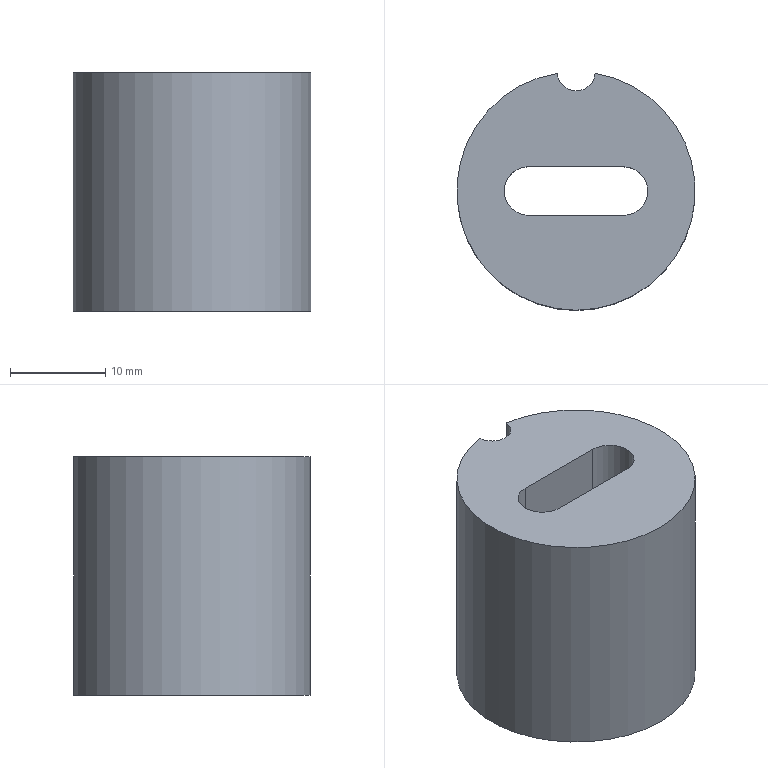Part | NX | features solid 2 | 1 solid | 10 faces | box 25 x 24.842 x 25 mm | volume 7869 mm3 | cylinder 5 | plane 5 | commonest cylinder face diameters 5.1 x2 4 x1 16.6 x1 25 x1
STEP:
#1=CARTESIAN_POINT('',(-200.99,448.658,32.));
#2=VERTEX_POINT('',#1);
#3=CARTESIAN_POINT('',(-200.99,448.658,57.));
#4=VERTEX_POINT('',#3);
#5=CARTESIAN_POINT('',(-200.99,448.658,44.5));
#6=DIRECTION('',(0.,0.,1.));
#7=VECTOR('',#6,1000.);
#8=LINE('',#5,#7);
#9=EDGE_CURVE('',#2,#4,#8,.T.);
#10=ORIENTED_EDGE('',*,*,#9,.T.);
#11=CARTESIAN_POINT('',(-204.978,448.663,57.));
#12=VERTEX_POINT('',#11);
#13=CARTESIAN_POINT('',(-202.998,436.321,57.));
#14=DIRECTION('',(0.,0.,-1.));
#15=DIRECTION('',(0.001167,1.,0.));
#16=AXIS2_PLACEMENT_3D('',#13,#14,#15);
#17=CIRCLE('',#16,12.5);
#18=EDGE_CURVE('',#4,#12,#17,.T.);
#19=ORIENTED_EDGE('',*,*,#18,.T.);
#20=CARTESIAN_POINT('',(-204.978,448.663,32.));
#21=VERTEX_POINT('',#20);
#22=CARTESIAN_POINT('',(-204.978,448.663,44.5));
#23=DIRECTION('',(0.,0.,1.));
#24=VECTOR('',#23,1000.);
#25=LINE('',#22,#24);
#26=EDGE_CURVE('',#12,#21,#25,.F.);
#27=ORIENTED_EDGE('',*,*,#26,.T.);
#28=CARTESIAN_POINT('',(-202.998,436.321,32.));
#29=DIRECTION('',(0.,0.,-1.));
#30=DIRECTION('',(0.001167,1.,0.));
#31=AXIS2_PLACEMENT_3D('',#28,#29,#30);
#32=CIRCLE('',#31,12.5);
#33=EDGE_CURVE('',#2,#21,#32,.T.);
#34=ORIENTED_EDGE('',*,*,#33,.F.);
#35=EDGE_LOOP('',(#10,#19,#27,#34));
#36=FACE_BOUND('',#35,.T.);
#37=CARTESIAN_POINT('',(-202.998,436.321,32.));
#38=DIRECTION('',(0.,0.,1.));
#39=DIRECTION('',(0.001167,1.,0.));
#40=AXIS2_PLACEMENT_3D('',#37,#38,#39);
#41=CYLINDRICAL_SURFACE('',#40,12.5);
#42=ADVANCED_FACE('',(#36),#41,.T.);
#43=CARTESIAN_POINT('',(-202.989,444.621,32.));
#44=VERTEX_POINT('',#43);
#45=CARTESIAN_POINT('',(-202.998,436.321,32.));
#46=DIRECTION('',(0.,0.,-1.));
#47=DIRECTION('',(0.001167,1.,0.));
#48=AXIS2_PLACEMENT_3D('',#45,#46,#47);
#49=CIRCLE('',#48,8.3);
#50=EDGE_CURVE('',#44,#44,#49,.T.);
#51=ORIENTED_EDGE('',*,*,#50,.F.);
#52=EDGE_LOOP('',(#51));
#53=FACE_BOUND('',#52,.T.);
#54=ORIENTED_EDGE('',*,*,#33,.T.);
#55=CARTESIAN_POINT('',(-202.984,448.821,32.));
#56=DIRECTION('',(0.,0.,-1.));
#57=DIRECTION('',(0.001167,1.,0.));
#58=AXIS2_PLACEMENT_3D('',#55,#56,#57);
#59=CIRCLE('',#58,2.);
#60=EDGE_CURVE('',#2,#21,#59,.T.);
#61=ORIENTED_EDGE('',*,*,#60,.F.);
#62=EDGE_LOOP('',(#54,#61));
#63=FACE_BOUND('',#62,.T.);
#64=CARTESIAN_POINT('',(-202.998,436.321,32.));
#65=DIRECTION('',(0.,0.,1.));
#66=DIRECTION('',(0.001167,1.,0.));
#67=AXIS2_PLACEMENT_3D('',#64,#65,#66);
#68=PLANE('',#67);
#69=ADVANCED_FACE('',(#53,#63),#68,.F.);
#70=CARTESIAN_POINT('',(-198.001,433.765,57.));
#71=VERTEX_POINT('',#70);
#72=CARTESIAN_POINT('',(-208.001,433.777,57.));
#73=VERTEX_POINT('',#72);
#74=CARTESIAN_POINT('',(-198.001,433.765,57.));
#75=DIRECTION('',(-1.,0.001167,0.));
#76=VECTOR('',#75,1000.);
#77=LINE('',#74,#76);
#78=EDGE_CURVE('',#71,#73,#77,.T.);
#79=ORIENTED_EDGE('',*,*,#78,.T.);
#80=CARTESIAN_POINT('',(-207.995,438.877,57.));
#81=VERTEX_POINT('',#80);
#82=CARTESIAN_POINT('',(-207.998,436.327,57.));
#83=DIRECTION('',(0.,0.,-1.));
#84=DIRECTION('',(0.001167,1.,0.));
#85=AXIS2_PLACEMENT_3D('',#82,#83,#84);
#86=CIRCLE('',#85,2.55);
#87=EDGE_CURVE('',#73,#81,#86,.T.);
#88=ORIENTED_EDGE('',*,*,#87,.T.);
#89=CARTESIAN_POINT('',(-197.995,438.865,57.));
#90=VERTEX_POINT('',#89);
#91=CARTESIAN_POINT('',(-197.995,438.865,57.));
#92=DIRECTION('',(-1.,0.001167,0.));
#93=VECTOR('',#92,1000.);
#94=LINE('',#91,#93);
#95=EDGE_CURVE('',#90,#81,#94,.T.);
#96=ORIENTED_EDGE('',*,*,#95,.F.);
#97=CARTESIAN_POINT('',(-197.998,436.315,57.));
#98=DIRECTION('',(0.,0.,-1.));
#99=DIRECTION('',(0.001167,1.,0.));
#100=AXIS2_PLACEMENT_3D('',#97,#98,#99);
#101=CIRCLE('',#100,2.55);
#102=EDGE_CURVE('',#90,#71,#101,.T.);
#103=ORIENTED_EDGE('',*,*,#102,.T.);
#104=EDGE_LOOP('',(#79,#88,#96,#103));
#105=FACE_BOUND('',#104,.T.);
#106=CARTESIAN_POINT('',(-202.984,448.821,57.));
#107=DIRECTION('',(0.,0.,-1.));
#108=DIRECTION('',(0.001167,1.,0.));
#109=AXIS2_PLACEMENT_3D('',#106,#107,#108);
#110=CIRCLE('',#109,2.);
#111=EDGE_CURVE('',#4,#12,#110,.T.);
#112=ORIENTED_EDGE('',*,*,#111,.T.);
#113=ORIENTED_EDGE('',*,*,#18,.F.);
#114=EDGE_LOOP('',(#112,#113));
#115=FACE_BOUND('',#114,.T.);
#116=CARTESIAN_POINT('',(-202.998,436.321,57.));
#117=DIRECTION('',(0.,0.,1.));
#118=DIRECTION('',(0.001167,1.,0.));
#119=AXIS2_PLACEMENT_3D('',#116,#117,#118);
#120=PLANE('',#119);
#121=ADVANCED_FACE('',(#105,#115),#120,.T.);
#122=ORIENTED_EDGE('',*,*,#50,.T.);
#123=EDGE_LOOP('',(#122));
#124=FACE_BOUND('',#123,.T.);
#125=CARTESIAN_POINT('',(-202.989,444.621,49.));
#126=VERTEX_POINT('',#125);
#127=CARTESIAN_POINT('',(-202.998,436.321,49.));
#128=DIRECTION('',(0.,0.,-1.));
#129=DIRECTION('',(0.001167,1.,0.));
#130=AXIS2_PLACEMENT_3D('',#127,#128,#129);
#131=CIRCLE('',#130,8.3);
#132=EDGE_CURVE('',#126,#126,#131,.T.);
#133=ORIENTED_EDGE('',*,*,#132,.F.);
#134=EDGE_LOOP('',(#133));
#135=FACE_BOUND('',#134,.T.);
#136=CARTESIAN_POINT('',(-202.998,436.321,32.));
#137=DIRECTION('',(0.,0.,1.));
#138=DIRECTION('',(0.001167,1.,0.));
#139=AXIS2_PLACEMENT_3D('',#136,#137,#138);
#140=CYLINDRICAL_SURFACE('',#139,8.3);
#141=ADVANCED_FACE('',(#124,#135),#140,.F.);
#142=CARTESIAN_POINT('',(-197.995,438.865,49.));
#143=VERTEX_POINT('',#142);
#144=CARTESIAN_POINT('',(-198.001,433.765,49.));
#145=VERTEX_POINT('',#144);
#146=CARTESIAN_POINT('',(-197.998,436.315,49.));
#147=DIRECTION('',(0.,0.,-1.));
#148=DIRECTION('',(0.001167,1.,0.));
#149=AXIS2_PLACEMENT_3D('',#146,#147,#148);
#150=CIRCLE('',#149,2.55);
#151=EDGE_CURVE('',#143,#145,#150,.T.);
#152=ORIENTED_EDGE('',*,*,#151,.F.);
#153=CARTESIAN_POINT('',(-207.995,438.877,49.));
#154=VERTEX_POINT('',#153);
#155=CARTESIAN_POINT('',(-202.995,438.871,49.));
#156=DIRECTION('',(-1.,0.001167,0.));
#157=VECTOR('',#156,1000.);
#158=LINE('',#155,#157);
#159=EDGE_CURVE('',#143,#154,#158,.T.);
#160=ORIENTED_EDGE('',*,*,#159,.T.);
#161=CARTESIAN_POINT('',(-208.001,433.777,49.));
#162=VERTEX_POINT('',#161);
#163=CARTESIAN_POINT('',(-207.998,436.327,49.));
#164=DIRECTION('',(0.,0.,-1.));
#165=DIRECTION('',(0.001167,1.,0.));
#166=AXIS2_PLACEMENT_3D('',#163,#164,#165);
#167=CIRCLE('',#166,2.55);
#168=EDGE_CURVE('',#162,#154,#167,.T.);
#169=ORIENTED_EDGE('',*,*,#168,.F.);
#170=CARTESIAN_POINT('',(-203.001,433.771,49.));
#171=DIRECTION('',(-1.,0.001167,0.));
#172=VECTOR('',#171,1000.);
#173=LINE('',#170,#172);
#174=EDGE_CURVE('',#145,#162,#173,.T.);
#175=ORIENTED_EDGE('',*,*,#174,.F.);
#176=EDGE_LOOP('',(#152,#160,#169,#175));
#177=FACE_BOUND('',#176,.T.);
#178=ORIENTED_EDGE('',*,*,#132,.T.);
#179=EDGE_LOOP('',(#178));
#180=FACE_BOUND('',#179,.T.);
#181=CARTESIAN_POINT('',(-202.998,436.321,49.));
#182=DIRECTION('',(0.,0.,1.));
#183=DIRECTION('',(0.001167,1.,0.));
#184=AXIS2_PLACEMENT_3D('',#181,#182,#183);
#185=PLANE('',#184);
#186=ADVANCED_FACE('',(#177,#180),#185,.F.);
#187=ORIENTED_EDGE('',*,*,#9,.F.);
#188=ORIENTED_EDGE('',*,*,#60,.T.);
#189=ORIENTED_EDGE('',*,*,#26,.F.);
#190=ORIENTED_EDGE('',*,*,#111,.F.);
#191=EDGE_LOOP('',(#187,#188,#189,#190));
#192=FACE_BOUND('',#191,.T.);
#193=CARTESIAN_POINT('',(-202.984,448.821,32.));
#194=DIRECTION('',(0.,0.,1.));
#195=DIRECTION('',(0.001167,1.,0.));
#196=AXIS2_PLACEMENT_3D('',#193,#194,#195);
#197=CYLINDRICAL_SURFACE('',#196,2.);
#198=ADVANCED_FACE('',(#192),#197,.F.);
#199=CARTESIAN_POINT('',(-198.001,433.765,32.));
#200=DIRECTION('',(0.,0.,1.));
#201=VECTOR('',#200,1000.);
#202=LINE('',#199,#201);
#203=EDGE_CURVE('',#145,#71,#202,.T.);
#204=ORIENTED_EDGE('',*,*,#203,.F.);
#205=ORIENTED_EDGE('',*,*,#174,.T.);
#206=CARTESIAN_POINT('',(-208.001,433.777,32.));
#207=DIRECTION('',(0.,0.,1.));
#208=VECTOR('',#207,1000.);
#209=LINE('',#206,#208);
#210=EDGE_CURVE('',#162,#73,#209,.T.);
#211=ORIENTED_EDGE('',*,*,#210,.T.);
#212=ORIENTED_EDGE('',*,*,#78,.F.);
#213=EDGE_LOOP('',(#204,#205,#211,#212));
#214=FACE_BOUND('',#213,.T.);
#215=CARTESIAN_POINT('',(-198.001,433.765,32.));
#216=DIRECTION('',(-0.001167,-1.,0.));
#217=DIRECTION('',(0.,0.,1.));
#218=AXIS2_PLACEMENT_3D('',#215,#216,#217);
#219=PLANE('',#218);
#220=ADVANCED_FACE('',(#214),#219,.F.);
#221=ORIENTED_EDGE('',*,*,#210,.F.);
#222=ORIENTED_EDGE('',*,*,#168,.T.);
#223=CARTESIAN_POINT('',(-207.995,438.877,32.));
#224=DIRECTION('',(0.,0.,1.));
#225=VECTOR('',#224,1000.);
#226=LINE('',#223,#225);
#227=EDGE_CURVE('',#154,#81,#226,.T.);
#228=ORIENTED_EDGE('',*,*,#227,.T.);
#229=ORIENTED_EDGE('',*,*,#87,.F.);
#230=EDGE_LOOP('',(#221,#222,#228,#229));
#231=FACE_BOUND('',#230,.T.);
#232=CARTESIAN_POINT('',(-207.998,436.327,32.));
#233=DIRECTION('',(0.,0.,1.));
#234=DIRECTION('',(0.001167,1.,0.));
#235=AXIS2_PLACEMENT_3D('',#232,#233,#234);
#236=CYLINDRICAL_SURFACE('',#235,2.55);
#237=ADVANCED_FACE('',(#231),#236,.F.);
#238=ORIENTED_EDGE('',*,*,#159,.F.);
#239=CARTESIAN_POINT('',(-197.995,438.865,32.));
#240=DIRECTION('',(0.,0.,1.));
#241=VECTOR('',#240,1000.);
#242=LINE('',#239,#241);
#243=EDGE_CURVE('',#143,#90,#242,.T.);
#244=ORIENTED_EDGE('',*,*,#243,.T.);
#245=ORIENTED_EDGE('',*,*,#95,.T.);
#246=ORIENTED_EDGE('',*,*,#227,.F.);
#247=EDGE_LOOP('',(#238,#244,#245,#246));
#248=FACE_BOUND('',#247,.T.);
#249=CARTESIAN_POINT('',(-197.995,438.865,32.));
#250=DIRECTION('',(-0.001167,-1.,0.));
#251=DIRECTION('',(0.,0.,1.));
#252=AXIS2_PLACEMENT_3D('',#249,#250,#251);
#253=PLANE('',#252);
#254=ADVANCED_FACE('',(#248),#253,.T.);
#255=ORIENTED_EDGE('',*,*,#243,.F.);
#256=ORIENTED_EDGE('',*,*,#151,.T.);
#257=ORIENTED_EDGE('',*,*,#203,.T.);
#258=ORIENTED_EDGE('',*,*,#102,.F.);
#259=EDGE_LOOP('',(#255,#256,#257,#258));
#260=FACE_BOUND('',#259,.T.);
#261=CARTESIAN_POINT('',(-197.998,436.315,32.));
#262=DIRECTION('',(0.,0.,1.));
#263=DIRECTION('',(0.001167,1.,0.));
#264=AXIS2_PLACEMENT_3D('',#261,#262,#263);
#265=CYLINDRICAL_SURFACE('',#264,2.55);
#266=ADVANCED_FACE('',(#260),#265,.F.);
#267=CLOSED_SHELL('',(#42,#69,#121,#141,#186,#198,#220,#237,#254,#266));
#268=MANIFOLD_SOLID_BREP('',#267);
#269=(LENGTH_UNIT()NAMED_UNIT(*)SI_UNIT(.MILLI.,.METRE.));
#270=UNCERTAINTY_MEASURE_WITH_UNIT(LENGTH_MEASURE(0.00001),#269,'','');
#271=(NAMED_UNIT(*)PLANE_ANGLE_UNIT()SI_UNIT($,.RADIAN.));
#272=(NAMED_UNIT(*)SI_UNIT($,.STERADIAN.)SOLID_ANGLE_UNIT());
#273=(GEOMETRIC_REPRESENTATION_CONTEXT(3)GLOBAL_UNCERTAINTY_ASSIGNED_CONTEXT((#270))GLOBAL_UNIT_ASSIGNED_CONTEXT((#269,#271,#272))REPRESENTATION_CONTEXT('',''));
#274=ADVANCED_BREP_SHAPE_REPRESENTATION('',(#268),#273);